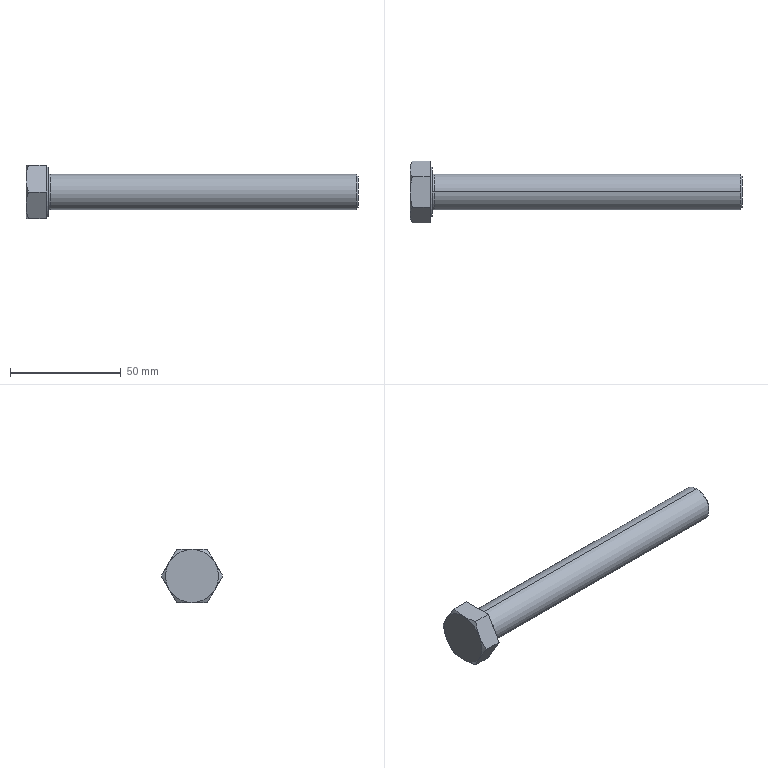Part | SolidWorks | features Chamfer 2, RevCut 2, Revolution 2, Extrusion 1, ICE 1 | 1 solid | 24 faces | box 150 x 27.713 x 24 mm | volume 33047 mm3 | cone 10 | plane 10 | cylinder 2 | torus 2 | commonest cylinder face diameters 16 x2
STEP:
#1=CARTESIAN_POINT('',(10.,0.,11.145));
#2=VERTEX_POINT('',#1);
#3=CARTESIAN_POINT('',(10.,0.,-11.145));
#4=VERTEX_POINT('',#3);
#5=CARTESIAN_POINT('',(10.,0.,0.));
#6=DIRECTION('',(-1.,0.,0.));
#7=DIRECTION('',(0.,0.,1.));
#8=AXIS2_PLACEMENT_3D('',#5,#6,#7);
#9=CIRCLE('',#8,11.145);
#10=EDGE_CURVE('',#2,#4,#9,.T.);
#11=ORIENTED_EDGE('',*,*,#10,.T.);
#12=CARTESIAN_POINT('',(9.2,0.,-11.945));
#13=VERTEX_POINT('',#12);
#14=CARTESIAN_POINT('',(9.2,0.,-11.945));
#15=DIRECTION('',(-0.7071,0.,-0.7071));
#16=VECTOR('',#15,1000.);
#17=LINE('',#14,#16);
#18=EDGE_CURVE('',#4,#13,#17,.T.);
#19=ORIENTED_EDGE('',*,*,#18,.T.);
#20=CARTESIAN_POINT('',(9.2,0.,11.945));
#21=VERTEX_POINT('',#20);
#22=CARTESIAN_POINT('',(9.2,0.,0.));
#23=DIRECTION('',(-1.,0.,0.));
#24=DIRECTION('',(0.,0.,1.));
#25=AXIS2_PLACEMENT_3D('',#22,#23,#24);
#26=CIRCLE('',#25,11.945);
#27=EDGE_CURVE('',#21,#13,#26,.T.);
#28=ORIENTED_EDGE('',*,*,#27,.F.);
#29=CARTESIAN_POINT('',(9.2,0.,11.945));
#30=DIRECTION('',(-0.7071,0.,0.7071));
#31=VECTOR('',#30,1000.);
#32=LINE('',#29,#31);
#33=EDGE_CURVE('',#2,#21,#32,.T.);
#34=ORIENTED_EDGE('',*,*,#33,.F.);
#35=EDGE_LOOP('',(#11,#19,#28,#34));
#36=FACE_OUTER_BOUND('',#35,.T.);
#37=CARTESIAN_POINT('',(9.2,0.,0.));
#38=DIRECTION('',(-1.,0.,0.));
#39=DIRECTION('',(0.,0.,1.));
#40=AXIS2_PLACEMENT_3D('',#37,#38,#39);
#41=CONICAL_SURFACE('',#40,11.945,0.7854);
#42=ADVANCED_FACE('',(#36),#41,.T.);
#43=CARTESIAN_POINT('',(150.,0.,-7.111));
#44=VERTEX_POINT('',#43);
#45=CARTESIAN_POINT('',(150.,0.,7.111));
#46=VERTEX_POINT('',#45);
#47=CARTESIAN_POINT('',(150.,0.,0.));
#48=DIRECTION('',(1.,0.,0.));
#49=DIRECTION('',(0.,0.,1.));
#50=AXIS2_PLACEMENT_3D('',#47,#48,#49);
#51=CIRCLE('',#50,7.111);
#52=EDGE_CURVE('',#44,#46,#51,.T.);
#53=ORIENTED_EDGE('',*,*,#52,.F.);
#54=CARTESIAN_POINT('',(149.111,0.,-8.));
#55=VERTEX_POINT('',#54);
#56=CARTESIAN_POINT('',(149.111,0.,-8.));
#57=DIRECTION('',(-0.7071,0.,-0.7071));
#58=VECTOR('',#57,1000.);
#59=LINE('',#56,#58);
#60=EDGE_CURVE('',#44,#55,#59,.T.);
#61=ORIENTED_EDGE('',*,*,#60,.T.);
#62=CARTESIAN_POINT('',(149.111,0.,8.));
#63=VERTEX_POINT('',#62);
#64=CARTESIAN_POINT('',(149.111,0.,0.));
#65=DIRECTION('',(-1.,0.,0.));
#66=DIRECTION('',(0.,0.,1.));
#67=AXIS2_PLACEMENT_3D('',#64,#65,#66);
#68=CIRCLE('',#67,8.);
#69=EDGE_CURVE('',#63,#55,#68,.T.);
#70=ORIENTED_EDGE('',*,*,#69,.F.);
#71=CARTESIAN_POINT('',(149.111,0.,8.));
#72=DIRECTION('',(-0.7071,0.,0.7071));
#73=VECTOR('',#72,1000.);
#74=LINE('',#71,#73);
#75=EDGE_CURVE('',#46,#63,#74,.T.);
#76=ORIENTED_EDGE('',*,*,#75,.F.);
#77=EDGE_LOOP('',(#53,#61,#70,#76));
#78=FACE_OUTER_BOUND('',#77,.T.);
#79=CARTESIAN_POINT('',(149.111,0.,0.));
#80=DIRECTION('',(-1.,0.,0.));
#81=DIRECTION('',(0.,0.,1.));
#82=AXIS2_PLACEMENT_3D('',#79,#80,#81);
#83=CONICAL_SURFACE('',#82,8.,0.7854);
#84=ADVANCED_FACE('',(#78),#83,.T.);
#85=ORIENTED_EDGE('',*,*,#69,.T.);
#86=CARTESIAN_POINT('',(10.85,0.,-8.));
#87=VERTEX_POINT('',#86);
#88=CARTESIAN_POINT('',(10.,0.,-8.));
#89=DIRECTION('',(-1.,0.,0.));
#90=VECTOR('',#89,1000.);
#91=LINE('',#88,#90);
#92=EDGE_CURVE('',#55,#87,#91,.T.);
#93=ORIENTED_EDGE('',*,*,#92,.T.);
#94=CARTESIAN_POINT('',(10.85,0.,8.));
#95=VERTEX_POINT('',#94);
#96=CARTESIAN_POINT('',(10.85,0.,0.));
#97=DIRECTION('',(-1.,0.,0.));
#98=DIRECTION('',(0.,0.,1.));
#99=AXIS2_PLACEMENT_3D('',#96,#97,#98);
#100=CIRCLE('',#99,8.);
#101=EDGE_CURVE('',#95,#87,#100,.T.);
#102=ORIENTED_EDGE('',*,*,#101,.F.);
#103=CARTESIAN_POINT('',(10.,0.,8.));
#104=DIRECTION('',(-1.,0.,0.));
#105=VECTOR('',#104,1000.);
#106=LINE('',#103,#105);
#107=EDGE_CURVE('',#63,#95,#106,.T.);
#108=ORIENTED_EDGE('',*,*,#107,.F.);
#109=EDGE_LOOP('',(#85,#93,#102,#108));
#110=FACE_OUTER_BOUND('',#109,.T.);
#111=CARTESIAN_POINT('',(10.,0.,0.));
#112=DIRECTION('',(-1.,0.,0.));
#113=DIRECTION('',(0.,0.,1.));
#114=AXIS2_PLACEMENT_3D('',#111,#112,#113);
#115=CYLINDRICAL_SURFACE('',#114,8.);
#116=ADVANCED_FACE('',(#110),#115,.T.);
#117=CARTESIAN_POINT('',(10.,0.,-8.85));
#118=VERTEX_POINT('',#117);
#119=CARTESIAN_POINT('',(10.,0.,8.85));
#120=VERTEX_POINT('',#119);
#121=CARTESIAN_POINT('',(10.,0.,0.));
#122=DIRECTION('',(-1.,0.,0.));
#123=DIRECTION('',(0.,0.,1.));
#124=AXIS2_PLACEMENT_3D('',#121,#122,#123);
#125=CIRCLE('',#124,8.85);
#126=EDGE_CURVE('',#118,#120,#125,.T.);
#127=ORIENTED_EDGE('',*,*,#126,.F.);
#128=CARTESIAN_POINT('',(10.85,0.,-8.85));
#129=DIRECTION('',(0.,1.,0.));
#130=DIRECTION('',(0.,0.,1.));
#131=AXIS2_PLACEMENT_3D('',#128,#129,#130);
#132=CIRCLE('',#131,0.85);
#133=EDGE_CURVE('',#118,#87,#132,.T.);
#134=ORIENTED_EDGE('',*,*,#133,.T.);
#135=CARTESIAN_POINT('',(10.85,0.,0.));
#136=DIRECTION('',(-1.,0.,0.));
#137=DIRECTION('',(0.,0.,1.));
#138=AXIS2_PLACEMENT_3D('',#135,#136,#137);
#139=CIRCLE('',#138,8.);
#140=EDGE_CURVE('',#87,#95,#139,.T.);
#141=ORIENTED_EDGE('',*,*,#140,.T.);
#142=CARTESIAN_POINT('',(10.85,0.,8.85));
#143=DIRECTION('',(0.,-1.,0.));
#144=DIRECTION('',(0.,0.,-1.));
#145=AXIS2_PLACEMENT_3D('',#142,#143,#144);
#146=CIRCLE('',#145,0.85);
#147=EDGE_CURVE('',#120,#95,#146,.T.);
#148=ORIENTED_EDGE('',*,*,#147,.F.);
#149=EDGE_LOOP('',(#127,#134,#141,#148));
#150=FACE_OUTER_BOUND('',#149,.T.);
#151=CARTESIAN_POINT('',(10.85,0.,0.));
#152=DIRECTION('',(-1.,0.,0.));
#153=DIRECTION('',(0.,0.,1.));
#154=AXIS2_PLACEMENT_3D('',#151,#152,#153);
#155=TOROIDAL_SURFACE('',#154,8.85,0.85);
#156=ADVANCED_FACE('',(#150),#155,.F.);
#157=CARTESIAN_POINT('',(10.,0.,0.));
#158=DIRECTION('',(-1.,0.,0.));
#159=DIRECTION('',(0.,0.,1.));
#160=AXIS2_PLACEMENT_3D('',#157,#158,#159);
#161=CIRCLE('',#160,8.85);
#162=EDGE_CURVE('',#120,#118,#161,.T.);
#163=ORIENTED_EDGE('',*,*,#162,.T.);
#164=ORIENTED_EDGE('',*,*,#126,.T.);
#165=EDGE_LOOP('',(#163,#164));
#166=FACE_BOUND('',#165,.T.);
#167=ORIENTED_EDGE('',*,*,#10,.F.);
#168=CARTESIAN_POINT('',(10.,0.,0.));
#169=DIRECTION('',(-1.,0.,0.));
#170=DIRECTION('',(0.,0.,1.));
#171=AXIS2_PLACEMENT_3D('',#168,#169,#170);
#172=CIRCLE('',#171,11.145);
#173=EDGE_CURVE('',#4,#2,#172,.T.);
#174=ORIENTED_EDGE('',*,*,#173,.F.);
#175=EDGE_LOOP('',(#167,#174));
#176=FACE_OUTER_BOUND('',#175,.T.);
#177=CARTESIAN_POINT('',(10.,6.928,-12.));
#178=DIRECTION('',(1.,0.,0.));
#179=DIRECTION('',(0.,0.,-1.));
#180=AXIS2_PLACEMENT_3D('',#177,#178,#179);
#181=PLANE('',#180);
#182=ADVANCED_FACE('',(#166,#176),#181,.T.);
#183=ORIENTED_EDGE('',*,*,#133,.F.);
#184=ORIENTED_EDGE('',*,*,#162,.F.);
#185=ORIENTED_EDGE('',*,*,#147,.T.);
#186=ORIENTED_EDGE('',*,*,#101,.T.);
#187=EDGE_LOOP('',(#183,#184,#185,#186));
#188=FACE_OUTER_BOUND('',#187,.T.);
#189=CARTESIAN_POINT('',(10.85,0.,0.));
#190=DIRECTION('',(-1.,0.,0.));
#191=DIRECTION('',(0.,0.,1.));
#192=AXIS2_PLACEMENT_3D('',#189,#190,#191);
#193=TOROIDAL_SURFACE('',#192,8.85,0.85);
#194=ADVANCED_FACE('',(#188),#193,.F.);
#195=CARTESIAN_POINT('',(150.,0.,0.));
#196=DIRECTION('',(1.,0.,0.));
#197=DIRECTION('',(0.,0.,1.));
#198=AXIS2_PLACEMENT_3D('',#195,#196,#197);
#199=CIRCLE('',#198,7.111);
#200=EDGE_CURVE('',#46,#44,#199,.T.);
#201=ORIENTED_EDGE('',*,*,#200,.T.);
#202=ORIENTED_EDGE('',*,*,#52,.T.);
#203=EDGE_LOOP('',(#201,#202));
#204=FACE_OUTER_BOUND('',#203,.T.);
#205=CARTESIAN_POINT('',(150.,8.,0.));
#206=DIRECTION('',(-1.,0.,0.));
#207=DIRECTION('',(0.,0.,1.));
#208=AXIS2_PLACEMENT_3D('',#205,#206,#207);
#209=PLANE('',#208);
#210=ADVANCED_FACE('',(#204),#209,.F.);
#211=ORIENTED_EDGE('',*,*,#92,.F.);
#212=CARTESIAN_POINT('',(149.111,0.,0.));
#213=DIRECTION('',(-1.,0.,0.));
#214=DIRECTION('',(0.,0.,1.));
#215=AXIS2_PLACEMENT_3D('',#212,#213,#214);
#216=CIRCLE('',#215,8.);
#217=EDGE_CURVE('',#55,#63,#216,.T.);
#218=ORIENTED_EDGE('',*,*,#217,.T.);
#219=ORIENTED_EDGE('',*,*,#107,.T.);
#220=ORIENTED_EDGE('',*,*,#140,.F.);
#221=EDGE_LOOP('',(#211,#218,#219,#220));
#222=FACE_OUTER_BOUND('',#221,.T.);
#223=CARTESIAN_POINT('',(10.,0.,0.));
#224=DIRECTION('',(-1.,0.,0.));
#225=DIRECTION('',(0.,0.,1.));
#226=AXIS2_PLACEMENT_3D('',#223,#224,#225);
#227=CYLINDRICAL_SURFACE('',#226,8.);
#228=ADVANCED_FACE('',(#222),#227,.T.);
#229=ORIENTED_EDGE('',*,*,#60,.F.);
#230=ORIENTED_EDGE('',*,*,#200,.F.);
#231=ORIENTED_EDGE('',*,*,#75,.T.);
#232=ORIENTED_EDGE('',*,*,#217,.F.);
#233=EDGE_LOOP('',(#229,#230,#231,#232));
#234=FACE_OUTER_BOUND('',#233,.T.);
#235=CARTESIAN_POINT('',(149.111,0.,0.));
#236=DIRECTION('',(-1.,0.,0.));
#237=DIRECTION('',(0.,0.,1.));
#238=AXIS2_PLACEMENT_3D('',#235,#236,#237);
#239=CONICAL_SURFACE('',#238,8.,0.7854);
#240=ADVANCED_FACE('',(#234),#239,.T.);
#241=ORIENTED_EDGE('',*,*,#27,.T.);
#242=CARTESIAN_POINT('',(9.2,0.,0.));
#243=DIRECTION('',(-1.,0.,0.));
#244=DIRECTION('',(0.,0.,1.));
#245=AXIS2_PLACEMENT_3D('',#242,#243,#244);
#246=CIRCLE('',#245,11.945);
#247=EDGE_CURVE('',#13,#21,#246,.T.);
#248=ORIENTED_EDGE('',*,*,#247,.T.);
#249=EDGE_LOOP('',(#241,#248));
#250=FACE_BOUND('',#249,.T.);
#251=CARTESIAN_POINT('',(9.2,-6.928,-12.));
#252=VERTEX_POINT('',#251);
#253=CARTESIAN_POINT('',(9.2,6.928,-12.));
#254=VERTEX_POINT('',#253);
#255=CARTESIAN_POINT('',(9.2,-6.928,-12.));
#256=DIRECTION('',(0.,1.,0.));
#257=VECTOR('',#256,1000.);
#258=LINE('',#255,#257);
#259=EDGE_CURVE('',#252,#254,#258,.T.);
#260=ORIENTED_EDGE('',*,*,#259,.T.);
#261=CARTESIAN_POINT('',(9.2,13.856,0.));
#262=VERTEX_POINT('',#261);
#263=CARTESIAN_POINT('',(9.2,6.928,-12.));
#264=DIRECTION('',(0.,0.5,0.866));
#265=VECTOR('',#264,1000.);
#266=LINE('',#263,#265);
#267=EDGE_CURVE('',#254,#262,#266,.T.);
#268=ORIENTED_EDGE('',*,*,#267,.T.);
#269=CARTESIAN_POINT('',(9.2,6.928,12.));
#270=VERTEX_POINT('',#269);
#271=CARTESIAN_POINT('',(9.2,13.856,0.));
#272=DIRECTION('',(0.,-0.5,0.866));
#273=VECTOR('',#272,1000.);
#274=LINE('',#271,#273);
#275=EDGE_CURVE('',#262,#270,#274,.T.);
#276=ORIENTED_EDGE('',*,*,#275,.T.);
#277=CARTESIAN_POINT('',(9.2,-6.928,12.));
#278=VERTEX_POINT('',#277);
#279=CARTESIAN_POINT('',(9.2,6.928,12.));
#280=DIRECTION('',(0.,-1.,0.));
#281=VECTOR('',#280,1000.);
#282=LINE('',#279,#281);
#283=EDGE_CURVE('',#270,#278,#282,.T.);
#284=ORIENTED_EDGE('',*,*,#283,.T.);
#285=CARTESIAN_POINT('',(9.2,-13.856,0.));
#286=VERTEX_POINT('',#285);
#287=CARTESIAN_POINT('',(9.2,-6.928,12.));
#288=DIRECTION('',(0.,-0.5,-0.866));
#289=VECTOR('',#288,1000.);
#290=LINE('',#287,#289);
#291=EDGE_CURVE('',#278,#286,#290,.T.);
#292=ORIENTED_EDGE('',*,*,#291,.T.);
#293=CARTESIAN_POINT('',(9.2,-13.856,0.));
#294=DIRECTION('',(0.,0.5,-0.866));
#295=VECTOR('',#294,1000.);
#296=LINE('',#293,#295);
#297=EDGE_CURVE('',#286,#252,#296,.T.);
#298=ORIENTED_EDGE('',*,*,#297,.T.);
#299=EDGE_LOOP('',(#260,#268,#276,#284,#292,#298));
#300=FACE_OUTER_BOUND('',#299,.T.);
#301=CARTESIAN_POINT('',(9.2,-11.945,0.));
#302=DIRECTION('',(1.,0.,0.));
#303=DIRECTION('',(0.,0.,-1.));
#304=AXIS2_PLACEMENT_3D('',#301,#302,#303);
#305=PLANE('',#304);
#306=ADVANCED_FACE('',(#250,#300),#305,.T.);
#307=ORIENTED_EDGE('',*,*,#18,.F.);
#308=ORIENTED_EDGE('',*,*,#173,.T.);
#309=ORIENTED_EDGE('',*,*,#33,.T.);
#310=ORIENTED_EDGE('',*,*,#247,.F.);
#311=EDGE_LOOP('',(#307,#308,#309,#310));
#312=FACE_OUTER_BOUND('',#311,.T.);
#313=CARTESIAN_POINT('',(9.2,0.,0.));
#314=DIRECTION('',(-1.,0.,0.));
#315=DIRECTION('',(0.,0.,1.));
#316=AXIS2_PLACEMENT_3D('',#313,#314,#315);
#317=CONICAL_SURFACE('',#316,11.945,0.7854);
#318=ADVANCED_FACE('',(#312),#317,.T.);
#319=CARTESIAN_POINT('',(0.,0.,-12.));
#320=VERTEX_POINT('',#319);
#321=CARTESIAN_POINT('',(0.,10.392,-6.));
#322=VERTEX_POINT('',#321);
#323=CARTESIAN_POINT('',(0.,0.,0.));
#324=DIRECTION('',(1.,0.,0.));
#325=DIRECTION('',(0.,0.,-1.));
#326=AXIS2_PLACEMENT_3D('',#323,#324,#325);
#327=CIRCLE('',#326,12.);
#328=EDGE_CURVE('',#320,#322,#327,.T.);
#329=ORIENTED_EDGE('',*,*,#328,.F.);
#330=CARTESIAN_POINT('',(0.,-10.392,-6.));
#331=VERTEX_POINT('',#330);
#332=CARTESIAN_POINT('',(0.,0.,0.));
#333=DIRECTION('',(1.,0.,0.));
#334=DIRECTION('',(0.,0.,-1.));
#335=AXIS2_PLACEMENT_3D('',#332,#333,#334);
#336=CIRCLE('',#335,12.);
#337=EDGE_CURVE('',#331,#320,#336,.T.);
#338=ORIENTED_EDGE('',*,*,#337,.F.);
#339=CARTESIAN_POINT('',(0.,-10.392,6.));
#340=VERTEX_POINT('',#339);
#341=CARTESIAN_POINT('',(0.,0.,0.));
#342=DIRECTION('',(1.,0.,0.));
#343=DIRECTION('',(0.,0.,-1.));
#344=AXIS2_PLACEMENT_3D('',#341,#342,#343);
#345=CIRCLE('',#344,12.);
#346=EDGE_CURVE('',#340,#331,#345,.T.);
#347=ORIENTED_EDGE('',*,*,#346,.F.);
#348=CARTESIAN_POINT('',(0.,0.,12.));
#349=VERTEX_POINT('',#348);
#350=CARTESIAN_POINT('',(0.,0.,0.));
#351=DIRECTION('',(1.,0.,0.));
#352=DIRECTION('',(0.,0.,-1.));
#353=AXIS2_PLACEMENT_3D('',#350,#351,#352);
#354=CIRCLE('',#353,12.);
#355=EDGE_CURVE('',#349,#340,#354,.T.);
#356=ORIENTED_EDGE('',*,*,#355,.F.);
#357=CARTESIAN_POINT('',(0.,10.392,6.));
#358=VERTEX_POINT('',#357);
#359=CARTESIAN_POINT('',(0.,0.,0.));
#360=DIRECTION('',(-1.,0.,0.));
#361=DIRECTION('',(0.,0.,1.));
#362=AXIS2_PLACEMENT_3D('',#359,#360,#361);
#363=CIRCLE('',#362,12.);
#364=EDGE_CURVE('',#349,#358,#363,.T.);
#365=ORIENTED_EDGE('',*,*,#364,.T.);
#366=CARTESIAN_POINT('',(0.,0.,0.));
#367=DIRECTION('',(1.,0.,0.));
#368=DIRECTION('',(0.,0.,-1.));
#369=AXIS2_PLACEMENT_3D('',#366,#367,#368);
#370=CIRCLE('',#369,12.);
#371=EDGE_CURVE('',#322,#358,#370,.T.);
#372=ORIENTED_EDGE('',*,*,#371,.F.);
#373=EDGE_LOOP('',(#329,#338,#347,#356,#365,#372));
#374=FACE_OUTER_BOUND('',#373,.T.);
#375=CARTESIAN_POINT('',(0.,6.928,-12.));
#376=DIRECTION('',(1.,0.,0.));
#377=DIRECTION('',(0.,0.,-1.));
#378=AXIS2_PLACEMENT_3D('',#375,#376,#377);
#379=PLANE('',#378);
#380=ADVANCED_FACE('',(#374),#379,.F.);
#381=CARTESIAN_POINT('',(1.072,6.928,-12.));
#382=VERTEX_POINT('',#381);
#383=CARTESIAN_POINT('',(0.,10.392,-6.));
#384=CARTESIAN_POINT('',(0.,10.098,-6.509));
#385=CARTESIAN_POINT('',(0.02533,9.803,-7.021));
#386=CARTESIAN_POINT('',(0.1234,9.219,-8.033));
#387=CARTESIAN_POINT('',(0.196,8.929,-8.535));
#388=CARTESIAN_POINT('',(0.476,8.063,-10.034));
#389=CARTESIAN_POINT('',(0.7454,7.493,-11.021));
#390=CARTESIAN_POINT('',(1.072,6.928,-12.));
#391=B_SPLINE_CURVE_WITH_KNOTS('',3,(#383,#384,#385,#386,#387,#388,#389,#390),.UNSPECIFIED.,.F.,.F.,(4,2,2,4),(0.00701,0.008756,0.0105,0.01399),.UNSPECIFIED.);
#392=EDGE_CURVE('',#322,#382,#391,.T.);
#393=ORIENTED_EDGE('',*,*,#392,.T.);
#394=CARTESIAN_POINT('',(1.072,6.928,-12.));
#395=CARTESIAN_POINT('',(0.7484,5.808,-12.));
#396=CARTESIAN_POINT('',(0.4791,4.673,-12.));
#397=CARTESIAN_POINT('',(0.1974,2.937,-12.));
#398=CARTESIAN_POINT('',(0.1238,2.353,-12.));
#399=CARTESIAN_POINT('',(0.0249,1.173,-12.));
#400=CARTESIAN_POINT('',(0.,0.5858,-12.));
#401=CARTESIAN_POINT('',(0.,0.,-12.));
#402=B_SPLINE_CURVE_WITH_KNOTS('',3,(#394,#395,#396,#397,#398,#399,#400,#401),.UNSPECIFIED.,.F.,.F.,(4,2,2,4),(0.005049,0.008547,0.0103,0.01204),.UNSPECIFIED.);
#403=EDGE_CURVE('',#382,#320,#402,.T.);
#404=ORIENTED_EDGE('',*,*,#403,.T.);
#405=ORIENTED_EDGE('',*,*,#328,.T.);
#406=EDGE_LOOP('',(#393,#404,#405));
#407=FACE_OUTER_BOUND('',#406,.T.);
#408=CARTESIAN_POINT('',(0.,0.,0.));
#409=DIRECTION('',(1.,0.,0.));
#410=DIRECTION('',(0.,0.,1.));
#411=AXIS2_PLACEMENT_3D('',#408,#409,#410);
#412=CONICAL_SURFACE('',#411,12.,1.047);
#413=ADVANCED_FACE('',(#407),#412,.T.);
#414=CARTESIAN_POINT('',(1.072,13.856,0.));
#415=VERTEX_POINT('',#414);
#416=CARTESIAN_POINT('',(0.,10.392,6.));
#417=CARTESIAN_POINT('',(0.,10.686,5.491));
#418=CARTESIAN_POINT('',(0.02533,10.982,4.979));
#419=CARTESIAN_POINT('',(0.1234,11.566,3.967));
#420=CARTESIAN_POINT('',(0.196,11.856,3.465));
#421=CARTESIAN_POINT('',(0.476,12.721,1.966));
#422=CARTESIAN_POINT('',(0.7454,13.291,0.9791));
#423=CARTESIAN_POINT('',(1.072,13.856,0.));
#424=B_SPLINE_CURVE_WITH_KNOTS('',3,(#416,#417,#418,#419,#420,#421,#422,#423),.UNSPECIFIED.,.F.,.F.,(4,2,2,4),(0.00701,0.008756,0.0105,0.01399),.UNSPECIFIED.);
#425=EDGE_CURVE('',#358,#415,#424,.T.);
#426=ORIENTED_EDGE('',*,*,#425,.T.);
#427=CARTESIAN_POINT('',(1.072,13.856,0.));
#428=CARTESIAN_POINT('',(0.7446,13.29,-0.9815));
#429=CARTESIAN_POINT('',(0.4751,12.719,-1.97));
#430=CARTESIAN_POINT('',(0.1021,11.565,-3.968));
#431=CARTESIAN_POINT('',(0.,10.982,-4.978));
#432=CARTESIAN_POINT('',(0.,10.392,-6.));
#433=B_SPLINE_CURVE_WITH_KNOTS('',3,(#427,#428,#429,#430,#431,#432),.UNSPECIFIED.,.F.,.F.,(4,2,4),(0.000000238,0.003505,0.00701),.UNSPECIFIED.);
#434=EDGE_CURVE('',#415,#322,#433,.T.);
#435=ORIENTED_EDGE('',*,*,#434,.T.);
#436=ORIENTED_EDGE('',*,*,#371,.T.);
#437=EDGE_LOOP('',(#426,#435,#436));
#438=FACE_OUTER_BOUND('',#437,.T.);
#439=CARTESIAN_POINT('',(0.,0.,0.));
#440=DIRECTION('',(1.,0.,0.));
#441=DIRECTION('',(0.,0.,1.));
#442=AXIS2_PLACEMENT_3D('',#439,#440,#441);
#443=CONICAL_SURFACE('',#442,12.,1.047);
#444=ADVANCED_FACE('',(#438),#443,.T.);
#445=CARTESIAN_POINT('',(1.072,6.928,12.));
#446=VERTEX_POINT('',#445);
#447=CARTESIAN_POINT('',(1.072,6.928,12.));
#448=CARTESIAN_POINT('',(0.7446,7.495,11.018));
#449=CARTESIAN_POINT('',(0.4751,8.066,10.03));
#450=CARTESIAN_POINT('',(0.1021,9.219,8.032));
#451=CARTESIAN_POINT('',(0.,9.802,7.022));
#452=CARTESIAN_POINT('',(0.,10.392,6.));
#453=B_SPLINE_CURVE_WITH_KNOTS('',3,(#447,#448,#449,#450,#451,#452),.UNSPECIFIED.,.F.,.F.,(4,2,4),(0.000000238,0.003505,0.00701),.UNSPECIFIED.);
#454=EDGE_CURVE('',#446,#358,#453,.T.);
#455=ORIENTED_EDGE('',*,*,#454,.T.);
#456=ORIENTED_EDGE('',*,*,#364,.F.);
#457=CARTESIAN_POINT('',(0.,0.,12.));
#458=CARTESIAN_POINT('',(0.,0.5858,12.));
#459=CARTESIAN_POINT('',(0.0249,1.173,12.));
#460=CARTESIAN_POINT('',(0.1238,2.353,12.));
#461=CARTESIAN_POINT('',(0.1974,2.937,12.));
#462=CARTESIAN_POINT('',(0.4791,4.673,12.));
#463=CARTESIAN_POINT('',(0.7484,5.808,12.));
#464=CARTESIAN_POINT('',(1.072,6.928,12.));
#465=B_SPLINE_CURVE_WITH_KNOTS('',3,(#457,#458,#459,#460,#461,#462,#463,#464),.UNSPECIFIED.,.F.,.F.,(4,2,2,4),(0.0194,0.02115,0.0229,0.02641),.UNSPECIFIED.);
#466=EDGE_CURVE('',#349,#446,#465,.T.);
#467=ORIENTED_EDGE('',*,*,#466,.T.);
#468=EDGE_LOOP('',(#455,#456,#467));
#469=FACE_OUTER_BOUND('',#468,.T.);
#470=CARTESIAN_POINT('',(0.,0.,0.));
#471=DIRECTION('',(1.,0.,0.));
#472=DIRECTION('',(0.,0.,1.));
#473=AXIS2_PLACEMENT_3D('',#470,#471,#472);
#474=CONICAL_SURFACE('',#473,12.,1.047);
#475=ADVANCED_FACE('',(#469),#474,.T.);
#476=CARTESIAN_POINT('',(1.072,-6.928,12.));
#477=VERTEX_POINT('',#476);
#478=CARTESIAN_POINT('',(1.072,-6.928,12.));
#479=CARTESIAN_POINT('',(0.7465,-5.801,12.));
#480=CARTESIAN_POINT('',(0.4737,-4.647,12.));
#481=CARTESIAN_POINT('',(0.1006,-2.334,12.));
#482=CARTESIAN_POINT('',(0.,-1.171,12.));
#483=CARTESIAN_POINT('',(0.,0.,12.));
#484=B_SPLINE_CURVE_WITH_KNOTS('',3,(#478,#479,#480,#481,#482,#483),.UNSPECIFIED.,.F.,.F.,(4,2,4),(0.01239,0.01589,0.0194),.UNSPECIFIED.);
#485=EDGE_CURVE('',#477,#349,#484,.T.);
#486=ORIENTED_EDGE('',*,*,#485,.T.);
#487=ORIENTED_EDGE('',*,*,#355,.T.);
#488=CARTESIAN_POINT('',(0.,-10.392,6.));
#489=CARTESIAN_POINT('',(0.,-10.098,6.509));
#490=CARTESIAN_POINT('',(0.02533,-9.803,7.021));
#491=CARTESIAN_POINT('',(0.1234,-9.219,8.033));
#492=CARTESIAN_POINT('',(0.196,-8.929,8.535));
#493=CARTESIAN_POINT('',(0.476,-8.063,10.034));
#494=CARTESIAN_POINT('',(0.7454,-7.493,11.021));
#495=CARTESIAN_POINT('',(1.072,-6.928,12.));
#496=B_SPLINE_CURVE_WITH_KNOTS('',3,(#488,#489,#490,#491,#492,#493,#494,#495),.UNSPECIFIED.,.F.,.F.,(4,2,2,4),(0.00701,0.008756,0.0105,0.01399),.UNSPECIFIED.);
#497=EDGE_CURVE('',#340,#477,#496,.T.);
#498=ORIENTED_EDGE('',*,*,#497,.T.);
#499=EDGE_LOOP('',(#486,#487,#498));
#500=FACE_OUTER_BOUND('',#499,.T.);
#501=CARTESIAN_POINT('',(0.,0.,0.));
#502=DIRECTION('',(1.,0.,0.));
#503=DIRECTION('',(0.,0.,1.));
#504=AXIS2_PLACEMENT_3D('',#501,#502,#503);
#505=CONICAL_SURFACE('',#504,12.,1.047);
#506=ADVANCED_FACE('',(#500),#505,.T.);
#507=CARTESIAN_POINT('',(1.072,-6.928,-12.));
#508=VERTEX_POINT('',#507);
#509=CARTESIAN_POINT('',(0.,0.,-12.));
#510=CARTESIAN_POINT('',(0.,-1.171,-12.));
#511=CARTESIAN_POINT('',(0.1006,-2.334,-12.));
#512=CARTESIAN_POINT('',(0.4737,-4.647,-12.));
#513=CARTESIAN_POINT('',(0.7465,-5.801,-12.));
#514=CARTESIAN_POINT('',(1.072,-6.928,-12.));
#515=B_SPLINE_CURVE_WITH_KNOTS('',3,(#509,#510,#511,#512,#513,#514),.UNSPECIFIED.,.F.,.F.,(4,2,4),(0.01204,0.01554,0.01904),.UNSPECIFIED.);
#516=EDGE_CURVE('',#320,#508,#515,.T.);
#517=ORIENTED_EDGE('',*,*,#516,.T.);
#518=CARTESIAN_POINT('',(1.072,-6.928,-12.));
#519=CARTESIAN_POINT('',(0.7446,-7.495,-11.018));
#520=CARTESIAN_POINT('',(0.4751,-8.066,-10.03));
#521=CARTESIAN_POINT('',(0.1021,-9.219,-8.032));
#522=CARTESIAN_POINT('',(0.,-9.802,-7.022));
#523=CARTESIAN_POINT('',(0.,-10.392,-6.));
#524=B_SPLINE_CURVE_WITH_KNOTS('',3,(#518,#519,#520,#521,#522,#523),.UNSPECIFIED.,.F.,.F.,(4,2,4),(0.000000238,0.003505,0.00701),.UNSPECIFIED.);
#525=EDGE_CURVE('',#508,#331,#524,.T.);
#526=ORIENTED_EDGE('',*,*,#525,.T.);
#527=ORIENTED_EDGE('',*,*,#337,.T.);
#528=EDGE_LOOP('',(#517,#526,#527));
#529=FACE_OUTER_BOUND('',#528,.T.);
#530=CARTESIAN_POINT('',(0.,0.,0.));
#531=DIRECTION('',(1.,0.,0.));
#532=DIRECTION('',(0.,0.,1.));
#533=AXIS2_PLACEMENT_3D('',#530,#531,#532);
#534=CONICAL_SURFACE('',#533,12.,1.047);
#535=ADVANCED_FACE('',(#529),#534,.T.);
#536=CARTESIAN_POINT('',(1.072,-13.856,0.));
#537=VERTEX_POINT('',#536);
#538=CARTESIAN_POINT('',(1.072,-13.856,0.));
#539=CARTESIAN_POINT('',(0.7446,-13.29,0.9815));
#540=CARTESIAN_POINT('',(0.4751,-12.719,1.97));
#541=CARTESIAN_POINT('',(0.1021,-11.565,3.968));
#542=CARTESIAN_POINT('',(0.,-10.982,4.978));
#543=CARTESIAN_POINT('',(0.,-10.392,6.));
#544=B_SPLINE_CURVE_WITH_KNOTS('',3,(#538,#539,#540,#541,#542,#543),.UNSPECIFIED.,.F.,.F.,(4,2,4),(0.000000238,0.003505,0.00701),.UNSPECIFIED.);
#545=EDGE_CURVE('',#537,#340,#544,.T.);
#546=ORIENTED_EDGE('',*,*,#545,.T.);
#547=ORIENTED_EDGE('',*,*,#346,.T.);
#548=CARTESIAN_POINT('',(0.,-10.392,-6.));
#549=CARTESIAN_POINT('',(0.,-10.686,-5.491));
#550=CARTESIAN_POINT('',(0.02533,-10.982,-4.979));
#551=CARTESIAN_POINT('',(0.1234,-11.566,-3.967));
#552=CARTESIAN_POINT('',(0.196,-11.856,-3.465));
#553=CARTESIAN_POINT('',(0.476,-12.721,-1.966));
#554=CARTESIAN_POINT('',(0.7454,-13.291,-0.9791));
#555=CARTESIAN_POINT('',(1.072,-13.856,0.));
#556=B_SPLINE_CURVE_WITH_KNOTS('',3,(#548,#549,#550,#551,#552,#553,#554,#555),.UNSPECIFIED.,.F.,.F.,(4,2,2,4),(0.00701,0.008756,0.0105,0.01399),.UNSPECIFIED.);
#557=EDGE_CURVE('',#331,#537,#556,.T.);
#558=ORIENTED_EDGE('',*,*,#557,.T.);
#559=EDGE_LOOP('',(#546,#547,#558));
#560=FACE_OUTER_BOUND('',#559,.T.);
#561=CARTESIAN_POINT('',(0.,0.,0.));
#562=DIRECTION('',(1.,0.,0.));
#563=DIRECTION('',(0.,0.,1.));
#564=AXIS2_PLACEMENT_3D('',#561,#562,#563);
#565=CONICAL_SURFACE('',#564,12.,1.047);
#566=ADVANCED_FACE('',(#560),#565,.T.);
#567=ORIENTED_EDGE('',*,*,#297,.F.);
#568=CARTESIAN_POINT('',(10.,-13.856,0.));
#569=DIRECTION('',(-1.,0.,0.));
#570=VECTOR('',#569,1000.);
#571=LINE('',#568,#570);
#572=EDGE_CURVE('',#286,#537,#571,.T.);
#573=ORIENTED_EDGE('',*,*,#572,.T.);
#574=ORIENTED_EDGE('',*,*,#557,.F.);
#575=ORIENTED_EDGE('',*,*,#525,.F.);
#576=CARTESIAN_POINT('',(10.,-6.928,-12.));
#577=DIRECTION('',(-1.,0.,0.));
#578=VECTOR('',#577,1000.);
#579=LINE('',#576,#578);
#580=EDGE_CURVE('',#252,#508,#579,.T.);
#581=ORIENTED_EDGE('',*,*,#580,.F.);
#582=EDGE_LOOP('',(#567,#573,#574,#575,#581));
#583=FACE_OUTER_BOUND('',#582,.T.);
#584=CARTESIAN_POINT('',(10.,-13.856,0.));
#585=DIRECTION('',(0.,0.866,0.5));
#586=DIRECTION('',(0.,-0.5,0.866));
#587=AXIS2_PLACEMENT_3D('',#584,#585,#586);
#588=PLANE('',#587);
#589=ADVANCED_FACE('',(#583),#588,.F.);
#590=ORIENTED_EDGE('',*,*,#291,.F.);
#591=CARTESIAN_POINT('',(10.,-6.928,12.));
#592=DIRECTION('',(-1.,0.,0.));
#593=VECTOR('',#592,1000.);
#594=LINE('',#591,#593);
#595=EDGE_CURVE('',#278,#477,#594,.T.);
#596=ORIENTED_EDGE('',*,*,#595,.T.);
#597=ORIENTED_EDGE('',*,*,#497,.F.);
#598=ORIENTED_EDGE('',*,*,#545,.F.);
#599=ORIENTED_EDGE('',*,*,#572,.F.);
#600=EDGE_LOOP('',(#590,#596,#597,#598,#599));
#601=FACE_OUTER_BOUND('',#600,.T.);
#602=CARTESIAN_POINT('',(10.,-6.928,12.));
#603=DIRECTION('',(0.,0.866,-0.5));
#604=DIRECTION('',(0.,0.5,0.866));
#605=AXIS2_PLACEMENT_3D('',#602,#603,#604);
#606=PLANE('',#605);
#607=ADVANCED_FACE('',(#601),#606,.F.);
#608=ORIENTED_EDGE('',*,*,#283,.F.);
#609=CARTESIAN_POINT('',(10.,6.928,12.));
#610=DIRECTION('',(-1.,0.,0.));
#611=VECTOR('',#610,1000.);
#612=LINE('',#609,#611);
#613=EDGE_CURVE('',#270,#446,#612,.T.);
#614=ORIENTED_EDGE('',*,*,#613,.T.);
#615=ORIENTED_EDGE('',*,*,#466,.F.);
#616=ORIENTED_EDGE('',*,*,#485,.F.);
#617=ORIENTED_EDGE('',*,*,#595,.F.);
#618=EDGE_LOOP('',(#608,#614,#615,#616,#617));
#619=FACE_OUTER_BOUND('',#618,.T.);
#620=CARTESIAN_POINT('',(10.,6.928,12.));
#621=DIRECTION('',(0.,0.,-1.));
#622=DIRECTION('',(0.,1.,0.));
#623=AXIS2_PLACEMENT_3D('',#620,#621,#622);
#624=PLANE('',#623);
#625=ADVANCED_FACE('',(#619),#624,.F.);
#626=ORIENTED_EDGE('',*,*,#275,.F.);
#627=CARTESIAN_POINT('',(10.,13.856,0.));
#628=DIRECTION('',(-1.,0.,0.));
#629=VECTOR('',#628,1000.);
#630=LINE('',#627,#629);
#631=EDGE_CURVE('',#262,#415,#630,.T.);
#632=ORIENTED_EDGE('',*,*,#631,.T.);
#633=ORIENTED_EDGE('',*,*,#425,.F.);
#634=ORIENTED_EDGE('',*,*,#454,.F.);
#635=ORIENTED_EDGE('',*,*,#613,.F.);
#636=EDGE_LOOP('',(#626,#632,#633,#634,#635));
#637=FACE_OUTER_BOUND('',#636,.T.);
#638=CARTESIAN_POINT('',(10.,13.856,0.));
#639=DIRECTION('',(0.,-0.866,-0.5));
#640=DIRECTION('',(0.,0.5,-0.866));
#641=AXIS2_PLACEMENT_3D('',#638,#639,#640);
#642=PLANE('',#641);
#643=ADVANCED_FACE('',(#637),#642,.F.);
#644=ORIENTED_EDGE('',*,*,#267,.F.);
#645=CARTESIAN_POINT('',(10.,6.928,-12.));
#646=DIRECTION('',(-1.,0.,0.));
#647=VECTOR('',#646,1000.);
#648=LINE('',#645,#647);
#649=EDGE_CURVE('',#254,#382,#648,.T.);
#650=ORIENTED_EDGE('',*,*,#649,.T.);
#651=ORIENTED_EDGE('',*,*,#392,.F.);
#652=ORIENTED_EDGE('',*,*,#434,.F.);
#653=ORIENTED_EDGE('',*,*,#631,.F.);
#654=EDGE_LOOP('',(#644,#650,#651,#652,#653));
#655=FACE_OUTER_BOUND('',#654,.T.);
#656=CARTESIAN_POINT('',(10.,6.928,-12.));
#657=DIRECTION('',(0.,-0.866,0.5));
#658=DIRECTION('',(0.,-0.5,-0.866));
#659=AXIS2_PLACEMENT_3D('',#656,#657,#658);
#660=PLANE('',#659);
#661=ADVANCED_FACE('',(#655),#660,.F.);
#662=ORIENTED_EDGE('',*,*,#259,.F.);
#663=ORIENTED_EDGE('',*,*,#580,.T.);
#664=ORIENTED_EDGE('',*,*,#516,.F.);
#665=ORIENTED_EDGE('',*,*,#403,.F.);
#666=ORIENTED_EDGE('',*,*,#649,.F.);
#667=EDGE_LOOP('',(#662,#663,#664,#665,#666));
#668=FACE_OUTER_BOUND('',#667,.T.);
#669=CARTESIAN_POINT('',(10.,-6.928,-12.));
#670=DIRECTION('',(0.,0.,1.));
#671=DIRECTION('',(0.,-1.,0.));
#672=AXIS2_PLACEMENT_3D('',#669,#670,#671);
#673=PLANE('',#672);
#674=ADVANCED_FACE('',(#668),#673,.F.);
#675=CLOSED_SHELL('',(#42,#84,#116,#156,#182,#194,#210,#228,#240,#306,#318,#380,#413,#444,#475,#506,#535,#566,#589,#607,#625,#643,#661,#674));
#676=MANIFOLD_SOLID_BREP('',#675);
#677=CARTESIAN_POINT('',(0.,0.,0.));
#678=DIRECTION('',(0.,0.,1.));
#679=DIRECTION('',(1.,0.,0.));
#680=AXIS2_PLACEMENT_3D('',#677,#678,#679);
#681=(LENGTH_UNIT()NAMED_UNIT(*)SI_UNIT(.MILLI.,.METRE.));
#682=UNCERTAINTY_MEASURE_WITH_UNIT(LENGTH_MEASURE(0.00001),#681,'','');
#683=(NAMED_UNIT(*)PLANE_ANGLE_UNIT()SI_UNIT($,.RADIAN.));
#684=(NAMED_UNIT(*)SI_UNIT($,.STERADIAN.)SOLID_ANGLE_UNIT());
#685=(GEOMETRIC_REPRESENTATION_CONTEXT(3)GLOBAL_UNCERTAINTY_ASSIGNED_CONTEXT((#682))GLOBAL_UNIT_ASSIGNED_CONTEXT((#681,#683,#684))REPRESENTATION_CONTEXT('',''));
#686=ADVANCED_BREP_SHAPE_REPRESENTATION('',(#676,#680),#685);